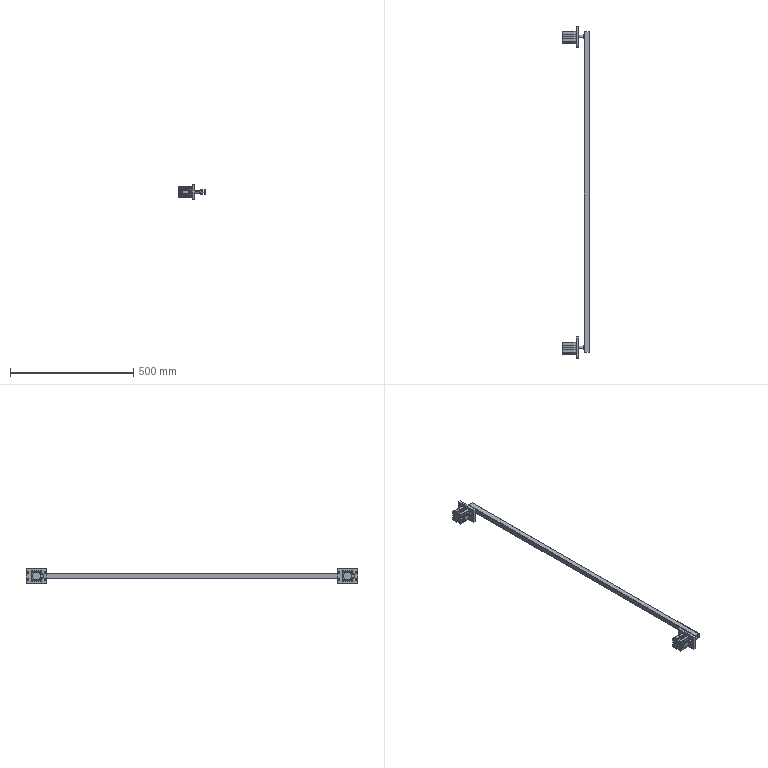Part | SolidWorks | 9 solids | 664 faces | box 108.5 x 1345 x 60 mm | volume 327193 mm3 | cylinder 308 | plane 228 | cone 124 | spline 4 | commonest cylinder face diameters 0.4 x92 4.917 x36 8.2 x32 0.8 x20 4.6 x16 6.6 x16